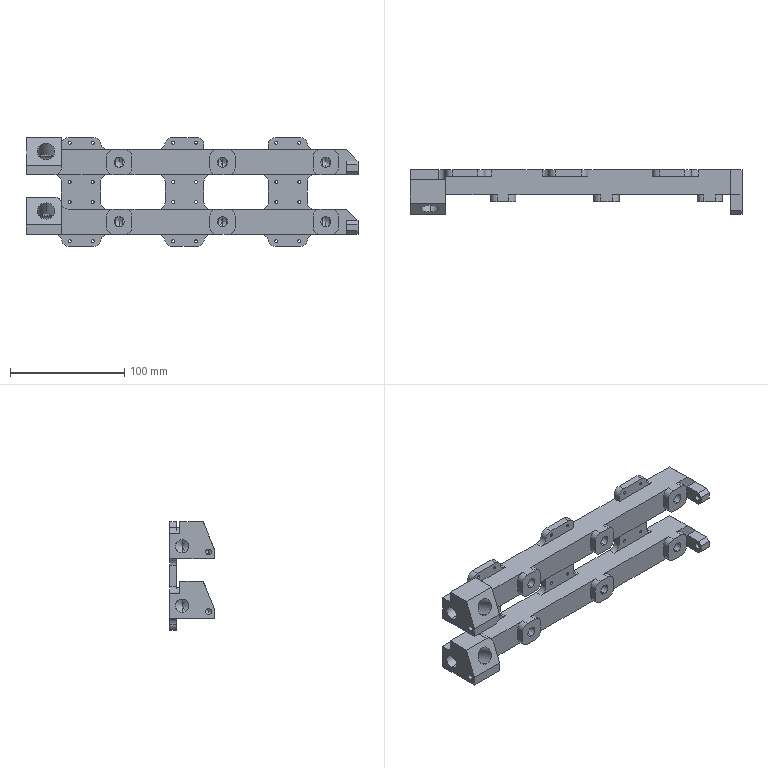NC program | NX | posted by the shop | part box 290 x 39.082 x 95 mm
Lines 26 to 834 of 5678:
(Adaptive-Milling, tool: D16)
N48 M6
N50 G54
N52 G17 G0 G90 X1.222 Y-63.601 S6000 M3
N54 G43 Z30. H0
N56 Z-39.
N58 G94 G1 X1.22 Y-63.551 Z-39.312 F3000.
N60 X1.219 Y-63.501 Z-39.436
N62 X1.218 Y-63.451 Z-39.527
N64 X1.216 Y-63.401 Z-39.6
N66 X1.215 Y-63.351 Z-39.661
N68 X1.214 Y-63.301 Z-39.714
N70 X1.212 Y-63.251 Z-39.76
N72 X1.211 Y-63.201 Z-39.8
N74 X1.209 Y-63.151 Z-39.835
N76 X1.208 Y-63.101 Z-39.866
N78 X1.207 Y-63.051 Z-39.893
N80 X1.205 Y-63.001 Z-39.917
N82 X1.204 Y-62.951 Z-39.937
N84 X1.203 Y-62.901 Z-39.954
N86 X1.201 Y-62.851 Z-39.968
N88 X1.2 Y-62.801 Z-39.98
N90 X1.198 Y-62.751 Z-39.989
N92 X1.197 Y-62.701 Z-39.995
N94 X1.196 Y-62.651 Z-39.999
N96 X1.194 Y-62.601 Z-40.
N98 X1.124 Y-60.047
N100 G3 X0.121 Y-58.596 R1.616
N102 X-2.756 Y-57.933 R10.574
N104 X-10.565 Y-57.551 R79.563
N106 X-23.969 Y-57.499 R842.44
N108 G1 X-143.716 Y-57.497
N110 G2 X-150.412 Y-54.647 R8.844
N112 X-153.599 Y-48.91 R13.945
N114 X-154.723 Y-41.889 R32.079
N116 X-154.983 Y-30.394 R194.097
N118 G1 X-154.996 Y-18.644
N120 Y46.304
N122 G2 X-152.083 Y52.973 R8.856
N124 X-146.325 Y56.123 R14.048
N126 X-139.426 Y57.22 R32.433
N128 X-128.931 Y57.479 R177.832
N130 G1 X-116.431 Y57.496
N132 X143.798
N134 G2 X150.38 Y54.674 R8.82
N136 X153.582 Y48.946 R13.912
N138 X154.719 Y41.927 R31.91
N140 X154.985 Y30.057 R196.37
N142 G1 X154.996 Y19.057
N144 X154.995 Y-46.398
N146 G2 X152.283 Y-52.775 R8.763
N148 X146.592 Y-56.038 R13.714
N150 X139.829 Y-57.19 R30.586
N152 X129.835 Y-57.476 R154.434
N154 G1 X117.71 Y-57.497
N156 X-11.965 Y-57.486
N158 G3 X-16.599 Y-56.761 R20.882
N160 X-26.006 Y-56.52 R167.041
N162 G1 X-37.716 Y-56.498
N164 X-140.466 Y-56.497
N166 G2 X-149.199 Y-52.31 R11.452
N168 X-152.55 Y-45.642 R17.207
N170 X-153.68 Y-38.24 R38.177
N172 X-153.974 Y-26.996 R188.105
N174 G1 X-153.995 Y-15.746
N176 X-153.996 Y42.841
N178 G2 X-153.526 Y46.171 R11.94
N180 G3 X-153.5 Y47.501 R9.579
N182 G1 X-153.395 Y48.831
N184 X-153.084 Y50.128
N186 X-152.573 Y51.36
N188 X-151.876 Y52.497
N190 X-151.01 Y53.511
N192 X-149.995 Y54.377
N194 X-148.858 Y55.074
N196 X-147.625 Y55.584
N198 X-146.329 Y55.895
N200 G2 X-142.608 Y56.081 R66.953
N202 X-124.249 Y56.484 R348.204
N204 G1 X-112.999 Y56.496
N206 X140.458 Y56.495
N208 G2 X149.223 Y52.273 R11.454
N210 X152.53 Y45.699 R17.19
N212 X153.702 Y37.925 R38.906
N214 X153.976 Y26.555 R200.993
N216 G1 X153.994 Y17.78
N218 X153.996 Y-42.833
N220 G2 X149.811 Y-51.692 R11.45
N222 X143.384 Y-54.978 R17.031
N224 X135.867 Y-56.171 R37.276
N226 X124.248 Y-56.48 R186.62
N228 G1 X113.248 Y-56.496
N230 X-11.927 Y-56.485
N232 G3 X-15.509 Y-56. R56.716
N234 G2 X-20.71 Y-55.788 R43.702
N236 G3 X-32.738 Y-55.51 R211.534
N238 G1 X-41.966 Y-55.498
N240 X-81.716
N242 G3 X-83.887 Y-55.893 R35.827
N244 G1 X-85.646 Y-56.
N246 X-107.835
N248 X-112.442 Y-55.682
N250 G3 X-123.727 Y-55.504 R282.665
N252 G1 X-129.467 Y-55.498
N254 G2 X-138.091 Y-55.47 R383.548
N256 X-148.481 Y-49.811 R13.286
N258 X-151.597 Y-42.762 R20.073
N260 G3 X-152.244 Y-41.447 R2.824
N262 G2 X-153.5 Y-36.999 R8.859
N264 G1 Y-4.499
N266 G3 X-153.038 Y5.415 R104.751
N268 G1 X-153.016 Y12.103
N270 G3 X-153.214 Y12.777 R3.314
N272 G1 X-153.461 Y14.041
N274 X-153.5 Y15.
N276 Y47.501
N278 X-153.395 Y48.831
N280 X-153.084 Y50.128
N282 X-152.573 Y51.36
N284 X-151.876 Y52.497
N286 X-151.01 Y53.511
N288 X-149.995 Y54.377
N290 X-148.858 Y55.074
N292 X-147.625 Y55.584
N294 X-146.329 Y55.895
N296 G2 X-144.749 Y56. R57.431
N298 G1 X-114.
N300 X-110.782 Y55.745
N302 G2 X-108.094 Y56. R16.841
N304 G1 X-85.645
N306 G2 X-81.287 Y55.694 R713.21
N308 G3 X-70.648 Y55.506 R248.45
N310 G1 X-62.415 Y55.496
N312 X-21.54 Y55.498
N314 G3 X-19.393 Y55.893 R85.483
N316 G1 X-17.634 Y56.
N318 X4.46
N320 G2 X8.837 Y55.693 R727.431
N322 G3 X20.222 Y55.502 R266.062
N324 G1 X26.71 Y55.496
N326 X68.835 Y55.504
N328 X70.901 Y55.893
N330 X72.66 Y56.
N332 X94.755
N334 G2 X99.091 Y55.695 R696.64
N336 G3 X109.726 Y55.505 R248.916
N338 G1 X118.46 Y55.496
N340 X137.085 Y55.494
N342 G2 X144.051 Y53.812 R13.906
N344 X149.84 Y47.579 R14.675
N346 X152.116 Y40.203 R24.995
N348 X152.867 Y30.74 R71.969
N350 G3 X153.033 Y29.778 R2.227
N352 G1 X153.383 Y28.408
N354 X153.5 Y26.999
N356 X153.498 Y17.083
N358 X153.5 Y14.776
N360 G3 X153.036 Y5.092 R95.967
N362 G1 X152.996 Y-6.586
N364 X153.003 Y-21.96
N366 G3 X153.404 Y-23.674 R35.017
N368 G1 X153.5 Y-25.
N370 Y-37.002
N372 G2 X153.046 Y-41.868 R93.667
N374 X146.881 Y-51.328 R13.741
N376 X139.617 Y-54.258 R21.35
N378 X130.811 Y-55.277 R52.766
N380 X115.939 Y-55.492 R356.297
N382 G1 X109.314 Y-55.495
N384 X98.594 Y-55.502
N386 X96.513 Y-55.893
N388 X94.754 Y-56.
N390 X72.565
N392 X67.934 Y-55.68
N394 G3 X56.4 Y-55.501 R289.681
N396 G1 X50.408 Y-55.496
N398 X8.409 Y-55.502
N400 X6.313 Y-55.893
N402 X4.554 Y-56.
N404 X-15.571
N406 G3 X-17.331 Y-57.76 R1.76
N408 X-15.569 Y-59.52 R1.76
N410 G1 X5.487 Y-59.487
N412 X8.652 Y-59.482 Z-39.9
N414 X68.036 Y-59.387
N416 X70.578 Y-59.379 Z-39.98
N418 G3 X71.182 Y-59.24 Z-40. R1.784
N420 X70.805 Y-55.893 R1.76
N422 G2 X68.041 Y-55.292 R22.211
N424 G3 X62.095 Y-54.676 R36.772
N426 X48.779 Y-54.5 R351.4
N428 G1 X43.284 Y-54.497
N430 X11.705 Y-54.499
N432 G3 X10.661 Y-54.623 R2.926
N434 G1 X9.728 Y-55.045
N436 X8.059 Y-55.569
N438 G3 X7.299 Y-58.449 R1.76
N440 X8.589 Y-59.009 Z-39.954 R1.774
N442 G1 X10.307 Y-59.005 Z-39.9
N444 X66.458 Y-58.903
N446 X67.375 Y-58.904 Z-39.929
N448 X68.292 Y-58.893 Z-39.958
N450 G3 X69.469 Y-58.346 Z-40. R1.759
N452 X68.714 Y-55.46 R1.76
N454 G2 X66.768 Y-54.786 R15.2
N456 G3 X61.979 Y-53.911 R21.369
N458 X51.6 Y-53.532 R135.121
N460 G1 X40.658 Y-53.497
N462 X14.929 Y-53.498
N464 G3 X12.662 Y-53.61 R17.193
N466 G1 X12.243 Y-53.763
N468 G2 X10.651 Y-54.627 R9.276
N470 G3 X9.899 Y-57.184 R1.76
N472 X11.369 Y-57.99 Z-39.945 R1.77
N474 G1 X12.786 Y-57.997 Z-39.9
N476 X64.859 Y-58.246
N478 X66.408 Y-58.248 Z-39.949
N480 G3 X67.77 Y-57.492 Z-40. R1.759
N482 X67.049 Y-54.89 R1.76
N484 X64.569 Y-53.838 R23.295
N486 X59.15 Y-52.916 R26.53
N488 X47.609 Y-52.527 R158.235
N490 G1 X36.659 Y-52.498
N492 X17.925 Y-52.499
N494 G3 X14.061 Y-52.692 R24.817
N496 X13.373 Y-52.978 R2.086
N498 G2 X12.199 Y-53.79 R6.674
N500 G3 X11.578 Y-56.152 R1.76
N502 X13.097 Y-57.053 Z-39.942 R1.77
N504 G1 X14.411 Y-57.066 Z-39.9
N506 X63.502 Y-57.565
N508 X64.227 Y-57.575 Z-39.923
N510 X64.951 Y-57.574 Z-39.946
N512 G3 X66.37 Y-56.738 Z-40. R1.759
N514 X65.785 Y-54.317 R1.76
N516 X61.719 Y-52.622 R10.968
N518 X54.751 Y-51.784 R43.548
N520 X41.639 Y-51.509 R266.83
N522 G1 X32.909 Y-51.498
N524 X20.429 Y-51.499
N526 G3 X15.695 Y-51.706 R35.54
N528 X14.322 Y-52.205 R2.598
N530 G1 X13.339 Y-53.004
N532 G3 X12.885 Y-55.227 R1.76
N534 X14.403 Y-56.145 Z-39.941 R1.768
N536 G1 X15.708 Y-56.166 Z-39.9
N538 X62.424 Y-56.907
N540 X63.149 Y-56.92 Z-39.923
N542 X63.874 Y-56.924 Z-39.946
N544 G3 X65.297 Y-56.097 Z-40. R1.759
N546 X64.717 Y-53.666 R1.76
N548 G2 X63.737 Y-53.003 R15.581
N550 G3 X60.216 Y-51.706 R12.37
N552 X52.864 Y-50.808 R46.008
N554 X40.254 Y-50.517 R250.806
N556 G1 X29.284 Y-50.499
N558 G3 X19.402 Y-50.551 R371.934
N560 X15.879 Y-50.988 R15.225
N562 X15.14 Y-51.379 R1.96
N564 G1 X14.261 Y-52.267
N566 G3 X13.968 Y-54.35 R1.76
N568 X15.473 Y-55.265 Z-39.942 R1.77
N570 G1 X16.793 Y-55.294 Z-39.9
N572 X61.531 Y-56.277
N574 X62.244 Y-56.295 Z-39.923
N576 X62.957 Y-56.303 Z-39.945
N578 G3 X64.397 Y-55.463 Z-40. R1.759
N580 X63.985 Y-53.166 R1.76
N582 X60.172 Y-51.133 R9.407
N584 X53.741 Y-50.023 R33.309
N586 X41.464 Y-49.545 R160.724
N588 X21.591 Y-49.539 R913.993
N590 X17.273 Y-49.958 R23.512
N592 X15.954 Y-50.487 R3.289
N594 X15.462 Y-51.054 R3.39
N596 G1 X15.11 Y-51.409
N598 G3 X14.827 Y-53.51 R1.76
N600 X16.315 Y-54.406 Z-39.943 R1.77
N602 G1 X17.662 Y-54.442 Z-39.9
N604 X60.641 Y-55.574
N606 X61.354 Y-55.594 Z-39.923
N608 X62.067 Y-55.605 Z-39.945
N610 G3 X63.51 Y-54.771 Z-40. R1.759
N612 X63.103 Y-52.468 R1.76
N614 X62.126 Y-51.631 R29.37
N616 X58.514 Y-50.084 R11.955
N618 X51.328 Y-48.973 R40.018
N620 X38.472 Y-48.54 R189.584
N622 X22.867 Y-48.556 R560.146
N624 X18.251 Y-49.017 R26.227
N626 X16.616 Y-49.644 R4.415
N628 G1 X16.389 Y-49.855
N630 X15.701 Y-50.744
N632 G3 X15.586 Y-52.73 R1.76
N634 X17.035 Y-53.58 Z-39.945 R1.77
N636 G1 X18.447 Y-53.627 Z-39.9
N638 X59.98 Y-54.992
N640 X60.703 Y-55.017 Z-39.923
N642 X61.425 Y-55.033 Z-39.946
N644 G3 X62.864 Y-54.226 Z-40. R1.759
N646 X62.633 Y-52.039 R1.76
N648 X59.421 Y-49.831 R7.907
N650 X53.287 Y-48.356 R26.234
N652 X42.607 Y-47.64 R100.888
N654 X24.477 Y-47.56 R476.924
N656 X19.135 Y-48.082 R29.78
N658 X17.238 Y-48.779 R6.156
N660 X16.54 Y-49.659 R2.333
N662 G1 X16.387 Y-49.857
N664 G3 X16.278 Y-51.853 R1.76
N666 X17.716 Y-52.693 Z-39.945 R1.77
N668 G1 X19.145 Y-52.745 Z-39.9
N670 X59.185 Y-54.187
N672 X59.907 Y-54.215 Z-39.923
N674 X60.628 Y-54.234 Z-39.946
N676 G3 X62.071 Y-53.43 Z-40. R1.759
N678 X61.842 Y-51.239 R1.76
N680 X61.021 Y-50.381 R13.833
N682 X57.589 Y-48.604 R10.794
N684 X50.608 Y-47.212 R33.569
N686 X38.296 Y-46.59 R137.151
N688 X27.135 Y-46.545 R869.367
N690 X20.636 Y-47.01 R42.298
N692 X17.81 Y-47.92 R8.824
N694 X17.27 Y-48.433 R2.081
N696 G1 X16.759 Y-49.292
N698 G3 X16.807 Y-51.168 R1.76
N700 X18.198 Y-51.951 Z-39.948 R1.771
N702 G1 X19.704 Y-52.013 Z-39.9
N704 X58.658 Y-53.632
N706 X60.138 Y-53.688 Z-39.947
N708 G3 X61.565 Y-52.924 Z-40. R1.759
N710 X61.504 Y-50.855 R1.76
N712 X58.951 Y-48.648 R6.645
N714 X53.758 Y-46.907 R19.421
N716 X45.109 Y-45.882 R60.777
N718 X26.51 Y-45.608 R264.181
N720 X20.757 Y-46.204 R32.916
N722 X18.084 Y-47.224 R7.939
N724 X17.442 Y-48.145 R1.976
N726 G1 X17.25 Y-48.467
N728 G3 X17.311 Y-50.363 R1.76
N730 X18.682 Y-51.125 Z-39.949 R1.773
N732 G1 X20.219 Y-51.196 Z-39.9
N734 X58.101 Y-52.933
N736 X59.594 Y-52.996 Z-39.947
N738 G3 X61.017 Y-52.25 Z-40. R1.759
N740 X60.969 Y-50.162 R1.76
N742 X58.008 Y-47.664 R7.327
N744 X52.138 Y-45.828 R22.377
N746 G1 X50.108 Y-45.5
N748 X22.233
N750 G3 X18.864 Y-46.276 R8.417
N752 X17.878 Y-47.155 R2.116
N754 G1 X17.576 Y-47.841
N756 G3 X18.129 Y-49.957 R1.76
N758 X19.873 Y-50.171 Z-39.942 R1.77
N760 G1 X21.092 Y-49.655 Z-39.9
N762 X21.552 Y-49.46
N764 X23.003 Y-48.84 Z-39.95
N766 G3 X23.952 Y-47.636 Z-40. R1.759
N768 X22.233 Y-45.5 R1.76
N770 X20.258 Y-45.527 R23.231
N772 X18.459 Y-46.204 R3.403
N774 X17.878 Y-47.155 R2.329
N776 X20.326 Y-49.413 R1.76
N778 G1 X21.444 Y-48.808
N780 G3 X20.608 Y-45.5 R1.76
N782 X19.437 Y-45.532 R10.983
N784 X18.07 Y-46.721 R1.795
N786 X19.541 Y-49.185 R1.76
N788 G1 X19.792 Y-49.205
N790 X22.946 Y-49.455 Z-39.9
N792 X57.538 Y-52.202
N794 X59.025 Y-52.315 Z-39.947
N796 G3 X60.474 Y-51.614 Z-40. R1.759
N798 X60.579 Y-49.658 R1.76
N800 X58.535 Y-47.483 R5.64
N802 X53.884 Y-45.511 R15.642
N804 G1 X50.011 Y-45.5
N806 G3 X48.436 Y-48.047 R1.76
N808 X49.496 Y-48.943 Z-39.955 R1.778
N810 G1 X51.158 Y-49.452 Z-39.9
N812 X56.884 Y-51.204
N814 X57.574 Y-51.417 Z-39.923
N816 X58.266 Y-51.62 Z-39.946
N818 G3 X59.868 Y-51.215 Z-40. R1.759
N820 X60.195 Y-49.013 R1.76
N822 X57.952 Y-46.628 R6.173
N824 X55.898 Y-45.558 R10.323
N826 G1 X55.549 Y-45.5
N828 X53.674
N830 G3 X51.944 Y-47.584 R1.76
N832 X52.973 Y-48.874 Z-39.946 R1.77
N834 G1 X54.301 Y-49.451 Z-39.9
N836 X56.382 Y-50.355
N838 X57.036 Y-50.641 Z-39.923
N840 X57.694 Y-50.918 Z-39.945
N842 G3 X59.343 Y-50.686 Z-40. R1.759
N844 X59.812 Y-48.369 R1.76
N846 X59.213 Y-47.363 R8.452
N848 X57.102 Y-45.626 R6.695
N850 X56.564 Y-45.5 R3.835
N852 G1 X55.439
N854 G3 X53.681 Y-47.34 R1.76
N856 X54.603 Y-48.809 Z-39.943 R1.77
N858 G1 X55.791 Y-49.45 Z-39.9
N860 X55.963 Y-49.543
N862 X56.59 Y-49.884 Z-39.923
N864 X57.222 Y-50.216 Z-39.945
N866 G3 X58.885 Y-50.125 Z-40. R1.759
N868 X59.576 Y-47.914 R1.76
N870 X57.868 Y-45.718 R4.353
N872 X57.147 Y-45.5 R2.125
N874 G1 X56.522
N876 G3 X55.548 Y-48.726 R1.76
N878 G1 X56.739 Y-49.518
N880 G3 X59.324 Y-47.342 R1.76
N882 X58.665 Y-46.109 R4.449
N884 X57.102 Y-45.5 R1.839
N886 X56.962 Y-49.014 R1.76
N888 X57.62 Y-49.023 R2.67
N890 X58.943 Y-46.493 R1.76
N892 X57.729 Y-45.544 R1.681
N894 X56.071 Y-46.236 R1.6
N896 G1 X55.7 Y-46.803
N898 X53.968 Y-49.452 Z-39.9
N900 X53.777 Y-49.747
N902 X53.576 Y-50.035
N904 G2 X52.694 Y-50.578 R1.604
N906 G1 X13.152 Y-59.545
N908 G2 X6.139 Y-60.595 R49.098
N910 X1.411 Y-60.803 R66.372
N912 G1 X-14.36 Y-60.928
N914 G2 X-15.666 Y-60.269 R1.601
N916 G1 X-15.887 Y-59.966
N918 X-17.749 Y-57.407 Z-40.
N920 X-18.119 Y-56.894
N922 X-18.501 Y-56.39
N924 G3 X-19.395 Y-55.893 R1.604
N926 G2 X-22.115 Y-55.306 R22.564
N928 G3 X-28.157 Y-54.683 R37.988
N930 X-41.472 Y-54.501 R350.861
N932 G1 X-46.966 Y-54.498
N934 X-77.347 Y-54.501
N936 G3 X-79.234 Y-54.538 R19.473
N938 X-80.472 Y-55.045 R6.456
N940 G1 X-82.141 Y-55.569
N942 G3 X-82.901 Y-58.449 R1.76
N944 X-81.611 Y-59.009 Z-39.954 R1.774
N946 G1 X-79.893 Y-59.005 Z-39.9
N948 X-23.742 Y-58.903
N950 X-22.825 Y-58.904 Z-39.929
N952 X-21.908 Y-58.893 Z-39.958
N954 G3 X-20.731 Y-58.346 Z-40. R1.759
N956 X-21.486 Y-55.46 R1.76
N958 G2 X-23.664 Y-54.716 R28.096
N960 G3 X-28.812 Y-53.867 R24.602
N962 X-40.008 Y-53.523 R164.268
N964 G1 X-49.467 Y-53.499
N966 X-74.954 Y-53.5
N968 G3 X-77.526 Y-53.608 R19.433
N970 G1 X-77.964 Y-53.767
N972 G2 X-79.549 Y-54.627 R9.223
N974 G3 X-80.303 Y-57.182 R1.76
N976 X-78.833 Y-57.99 Z-39.945 R1.77
N978 G1 X-77.417 Y-57.998 Z-39.9
N980 X-25.23 Y-58.296
N982 X-23.68 Y-58.3 Z-39.949
N984 G3 X-22.318 Y-57.546 Z-40. R1.759
N986 X-23.038 Y-54.941 R1.76
N988 X-25.593 Y-53.855 R24.387
N990 X-31.096 Y-52.918 R26.592
N992 X-42.642 Y-52.529 R159.475
N994 G1 X-53.591 Y-52.5
N996 X-72.329
N998 G3 X-76.143 Y-52.69 R24.466
N1000 X-76.829 Y-52.979 R2.071
N1002 G2 X-78.001 Y-53.79 R6.668
N1004 G3 X-78.622 Y-56.152 R1.76
N1006 X-77.103 Y-57.053 Z-39.942 R1.77
N1008 G1 X-75.789 Y-57.066 Z-39.9
N1010 X-26.698 Y-57.565
N1012 X-25.973 Y-57.575 Z-39.923
N1014 X-25.249 Y-57.574 Z-39.946
N1016 G3 X-23.83 Y-56.738 Z-40. R1.759
N1018 X-24.415 Y-54.317 R1.76
N1020 X-28.515 Y-52.619 R11.014
N1022 X-35.847 Y-51.767 R46.047
N1024 X-48.86 Y-51.511 R279.995
N1026 G1 X-57.091 Y-51.5
N1028 X-69.821
N1030 G3 X-74.454 Y-51.694 R37.434
N1032 X-75.745 Y-52.102 R2.868
N1034 G1 X-76.861 Y-53.004
N1036 G3 X-77.315 Y-55.227 R1.76
N1038 X-75.797 Y-56.145 Z-39.941 R1.768
N1040 G1 X-74.492 Y-56.166 Z-39.9
N1042 X-27.776 Y-56.907
N1044 X-27.051 Y-56.92 Z-39.923
N1046 X-26.326 Y-56.924 Z-39.946
N1048 G3 X-24.903 Y-56.097 Z-40. R1.759
N1050 X-25.483 Y-53.666 R1.76
N1052 G2 X-26.475 Y-52.998 R17.673
N1054 G3 X-30.03 Y-51.707 R12.304
N1056 X-37.385 Y-50.81 R46.137
N1058 X-49.748 Y-50.52 R247.617
N1060 G1 X-60.716 Y-50.5
N1062 G3 X-70.96 Y-50.557 R352.894
N1064 X-74.413 Y-51.014 R13.98
N1066 X-75.061 Y-51.38 R2.092
N1068 G1 X-75.941 Y-52.269
N1070 G3 X-76.233 Y-54.352 R1.76
N1072 X-74.728 Y-55.266 Z-39.942 R1.77
N1074 G1 X-73.408 Y-55.295 Z-39.9
N1076 X-28.669 Y-56.277
N1078 X-27.956 Y-56.295 Z-39.923
N1080 X-27.243 Y-56.303 Z-39.945
N1082 G3 X-25.803 Y-55.463 Z-40. R1.759
N1084 X-26.215 Y-53.166 R1.76
N1086 X-29.81 Y-51.207 R9.157
N1088 X-36.283 Y-50.044 R32.125
N1090 X-47.678 Y-49.56 R147.388
N1092 X-68.429 Y-49.535 R947.944
N1094 X-72.881 Y-49.948 R24.433
N1096 X-74.16 Y-50.419 R3.602
N1098 X-74.738 Y-51.054 R2.735
N1100 G1 X-75.09 Y-51.409
N1102 G3 X-75.373 Y-53.51 R1.76
N1104 X-73.885 Y-54.406 Z-39.943 R1.77
N1106 G1 X-72.538 Y-54.442 Z-39.9
N1108 X-29.559 Y-55.574
N1110 X-28.846 Y-55.594 Z-39.923
N1112 X-28.133 Y-55.605 Z-39.945
N1114 G3 X-26.69 Y-54.771 Z-40. R1.759
N1116 X-27.097 Y-52.468 R1.76
N1118 G1 X-27.826 Y-51.819
N1120 G3 X-31.282 Y-50.205 R10.652
N1122 X-38.125 Y-49.041 R36.074
N1124 X-50.419 Y-48.555 R163.69
N1126 X-67.151 Y-48.55 R638.118
N1128 X-71.823 Y-48.989 R27.96
N1130 X-73.496 Y-49.576 R5.152
N1132 G1 X-73.802 Y-49.844
N1134 X-74.491 Y-50.734
N1136 G3 X-74.606 Y-52.72 R1.76
N1138 X-73.157 Y-53.57 Z-39.945 R1.77
N1140 G1 X-71.744 Y-53.617 Z-39.9
N1142 X-30.22 Y-54.991
N1144 X-29.498 Y-55.017 Z-39.923
N1146 X-28.775 Y-55.033 Z-39.946
N1148 G3 X-27.336 Y-54.226 Z-40. R1.759
N1150 X-27.567 Y-52.039 R1.76
N1152 X-30.965 Y-49.763 R8.15
N1154 X-36.956 Y-48.354 R26.561
N1156 X-47.643 Y-47.641 R101.61
N1158 X-65.771 Y-47.562 R474.164
N1160 X-70.841 Y-48.034 R31.056
N1162 X-72.896 Y-48.729 R7.396
N1164 X-73.66 Y-49.659 R2.443
N1166 G1 X-73.813 Y-49.857
N1168 G3 X-73.923 Y-51.851 R1.76
N1170 X-72.487 Y-52.693 Z-39.945 R1.77
N1172 G1 X-71.057 Y-52.747 Z-39.9
N1174 X-30.93 Y-54.273
N1176 X-30.209 Y-54.303 Z-39.923
N1178 X-29.487 Y-54.323 Z-39.946
N1180 G3 X-28.043 Y-53.521 Z-40. R1.759
N1182 X-28.27 Y-51.328 R1.76
N1184 X-29.169 Y-50.392 R19.909
N1186 X-32.507 Y-48.643 R10.573
N1188 X-39.192 Y-47.261 R32.278
N1190 X-51.341 Y-46.602 R128.298
N1192 X-63.468 Y-46.553 R704.361
N1194 X-69.509 Y-47.002 R41.449
N1196 X-72.376 Y-47.905 R9.1
N1198 X-72.919 Y-48.415 R2.1
N1200 G1 X-73.431 Y-49.275
N1202 G3 X-73.382 Y-51.151 R1.76
N1204 X-71.992 Y-51.933 Z-39.948 R1.771
N1206 G1 X-70.484 Y-51.996 Z-39.9
N1208 X-31.542 Y-53.632
N1210 X-30.063 Y-53.688 Z-39.947
N1212 G3 X-28.635 Y-52.925 Z-40. R1.759
N1214 X-28.696 Y-50.855 R1.76
N1216 X-31.275 Y-48.636 R6.662
N1218 X-36.893 Y-46.821 R20.822
N1220 X-46.202 Y-45.823 R68.664
N1222 X-63.851 Y-45.616 R267.848
N1224 X-69.478 Y-46.212 R32.459
N1226 X-72.13 Y-47.233 R7.706
N1228 X-72.758 Y-48.145 R1.994
N1230 G1 X-72.95 Y-48.467
N1232 G3 X-72.889 Y-50.363 R1.76
N1234 X-71.518 Y-51.125 Z-39.949 R1.773
N1236 G1 X-69.981 Y-51.196 Z-39.9
N1238 X-32.099 Y-52.933
N1240 X-30.606 Y-52.996 Z-39.947
N1242 G3 X-29.183 Y-52.25 Z-40. R1.759
N1244 X-29.231 Y-50.162 R1.76
N1246 X-31.865 Y-47.841 R6.959
N1248 X-37.478 Y-45.949 R20.618
N1250 X-40.132 Y-45.5 R59.726
N1252 G1 X-68.175 Y-45.513
N1254 G3 X-71.649 Y-46.448 R7.718
N1256 X-72.326 Y-47.165 R1.84
N1258 G1 X-72.629 Y-47.851
N1260 G3 X-72.085 Y-49.961 R1.76
N1262 X-70.344 Y-50.187 Z-39.942 R1.77
N1264 G1 X-69.118 Y-49.678 Z-39.9
N1266 X-68.591 Y-49.46
N1268 X-67.124 Y-48.846 Z-39.95
N1270 G3 X-66.168 Y-47.662 Z-40. R1.759
N1272 X-67.882 Y-45.5 R1.76
N1274 X-69.935 Y-45.524 R28.585
N1276 X-71.717 Y-46.179 R3.457
N1278 X-72.36 Y-47.241 R2.727
N1280 X-69.824 Y-49.448 R1.76
N1282 G1 X-68.706 Y-48.757
N1284 G3 X-69.632 Y-45.5 R1.76
N1286 X-70.763 Y-45.532 R10.852
N1288 X-72.13 Y-46.721 R1.795
N1290 X-70.659 Y-49.185 R1.76
N1292 G1 X-70.408 Y-49.205
N1294 X-67.254 Y-49.455 Z-39.9
N1296 X-32.662 Y-52.202
N1298 X-31.175 Y-52.315 Z-39.947
N1300 G3 X-29.726 Y-51.614 Z-40. R1.759
N1302 X-29.621 Y-49.658 R1.76
N1304 X-31.815 Y-47.391 R5.887
N1306 X-36.353 Y-45.508 R15.701
N1308 G1 X-40.195 Y-45.5
N1310 G3 X-41.791 Y-48.002 R1.76
N1312 X-40.725 Y-48.938 Z-39.954 R1.773
N1314 G1 X-39.099 Y-49.452 Z-39.9
N1316 X-33.261 Y-51.296
N1318 X-32.574 Y-51.514 Z-39.923
N1320 X-31.885 Y-51.724 Z-39.946
N1322 G3 X-30.278 Y-51.331 Z-40. R1.759
N1324 X-29.941 Y-49.121 R1.76
N1326 X-32.273 Y-46.615 R6.291
N1328 X-34.332 Y-45.553 R9.809
N1330 G1 X-34.651 Y-45.5
N1332 X-36.526
N1334 G3 X-38.256 Y-47.584 R1.76
N1336 X-37.227 Y-48.874 Z-39.946 R1.77
N1338 G1 X-35.9 Y-49.451 Z-39.9
N1340 X-33.818 Y-50.355
N1342 X-33.164 Y-50.641 Z-39.923
N1344 X-32.506 Y-50.918 Z-39.945
N1346 G3 X-30.857 Y-50.686 Z-40. R1.759
N1348 X-30.388 Y-48.369 R1.76
N1350 X-30.99 Y-47.361 R8.305
N1352 X-33.15 Y-45.613 R6.41
N1354 X-33.645 Y-45.5 R7.782
N1356 G1 X-34.77
N1358 G3 X-36.528 Y-47.343 R1.76
N1360 X-35.604 Y-48.81 Z-39.943 R1.77
N1362 G1 X-34.413 Y-49.45 Z-39.9
N1364 X-34.236 Y-49.546
N1366 X-33.608 Y-49.886 Z-39.923
N1368 X-32.975 Y-50.217 Z-39.945
N1370 G3 X-31.313 Y-50.124 Z-40. R1.759
N1372 X-30.624 Y-47.914 R1.76
N1374 X-32.343 Y-45.716 R4.342
N1376 X-33.06 Y-45.5 R2.139
N1378 G1 X-33.685
N1380 G3 X-34.655 Y-48.728 R1.76
N1382 G1 X-33.457 Y-49.52
N1384 G3 X-30.876 Y-47.342 R1.76
N1386 X-31.696 Y-45.956 R3.954
N1388 X-33.098 Y-45.5 R1.858
N1390 X-33.669 Y-48.925 R1.76
N1392 G1 X-33.418 Y-49.01
N1394 X-33.164 Y-49.086
N1396 G3 X-31.178 Y-46.656 R1.76
N1398 X-32.586 Y-45.521 R1.758
N1400 X-34. Y-46.186 R1.601
N1402 G1 X-34.494 Y-46.878
N1404 X-36.334 Y-49.452 Z-39.9
N1406 X-36.557 Y-49.769
N1408 X-36.795 Y-50.076
N1410 G2 X-37.62 Y-50.556 R1.606
N1412 G1 X-77.163 Y-59.523
N1414 G2 X-84.176 Y-60.575 R49.295
N1416 X-88.904 Y-60.787 R66.833
N1418 G1 X-104.56 Y-60.928
N1420 G2 X-105.868 Y-60.269 R1.601
N1422 G1 X-106.089 Y-59.965
N1424 X-107.95 Y-57.406 Z-40.
N1426 X-108.319 Y-56.893
N1428 X-108.701 Y-56.39
N1430 G3 X-109.595 Y-55.893 R1.604
N1432 G2 X-112.343 Y-55.296 R21.655
N1434 G3 X-118.281 Y-54.678 R36.613
N1436 X-131.596 Y-54.501 R351.169
N1438 G2 X-136.591 Y-54.388 R56.282
N1440 X-147.561 Y-47.771 R14.554
N1442 X-149.504 Y-44.354 R46.844
N1444 G3 X-149.863 Y-43.971 R3.099
N1446 G2 X-151.555 Y-42.411 R9.77
N1448 G1 X-151.919 Y-41.902
N1450 G3 X-154.503 Y-41.876 R1.6
N1452 X-154.791 Y-43.175 Z-39.957 R1.678
N1454 G1 X-154.572 Y-44.957 Z-39.9
N1456 X-154.218 Y-47.844
N1458 G3 X-153.762 Y-48.78 R1.604
N1460 G1 X-148.167 Y-54.375
N1462 G3 X-144.454 Y-57.032 R14.335
N1464 X-139.781 Y-58.694 R19.135
N1466 X-137.554 Y-59.003 R17.199
N1468 G1 X-116.721 Y-60.495
N1470 G3 X-115.974 Y-60.369 R1.615
N1472 G1 X-113.159 Y-59.157
N1474 X-111.454 Y-58.418 Z-39.959
N1476 G3 X-110.633 Y-57.449 Z-40. R1.6
N1478 X-111.686 Y-55.46 R1.6
N1480 G2 X-113.841 Y-54.721 R25.579
N1482 G3 X-118.944 Y-53.867 R23.876
N1484 X-128.776 Y-53.534 R146.543
N1486 G2 X-134.256 Y-53.398 R76.692
N1488 X-145.17 Y-47.951 R15.791
N1490 G3 X-147.511 Y-45.243 R118.595
N1492 G1 X-147.873 Y-45.
N1494 G2 X-149.863 Y-43.971 R9.861
N1496 G3 X-152.087 Y-44.561 R1.6
N1498 X-152.186 Y-45.91 Z-39.956 R1.612
N1500 G1 X-151.557 Y-47.562 Z-39.9
N1502 X-150.922 Y-49.232
N1504 G3 X-149.863 Y-50.202 R1.601
N1506 G1 X-117.643 Y-59.347
N1508 G3 X-116.579 Y-59.28 R1.604
N1510 G1 X-114.877 Y-58.554
N1512 X-113.192 Y-57.831 Z-39.958
N1514 G3 X-112.361 Y-56.842 Z-40. R1.6
N1516 X-113.238 Y-54.941 R1.6
N1518 X-115.896 Y-53.818 R23.517
N1520 X-121.445 Y-52.899 R27.382
N1522 X-130.373 Y-52.533 R170.135
N1524 G2 X-136.649 Y-51.55 R22.314
N1526 X-142.989 Y-47.858 R18.914
N1528 G3 X-145.683 Y-45.615 R45.331
N1530 X-146.793 Y-45.309 R2.868
N1532 G1 X-147.987 Y-44.95
N1534 G3 X-149.163 Y-48.259 R-1.76
N1536 G1 X-147.938 Y-48.601
N1538 X-144.89 Y-49.452 Z-39.9
N1540 X-117.799 Y-57.014
N1542 X-115.914 Y-57.535 Z-39.962
N1544 G3 X-114.738 Y-57.39 Z-40. R1.76
N1546 X-114.615 Y-54.317 R1.76
N1548 X-118.661 Y-52.626 R10.935
N1550 X-125.283 Y-51.806 R42.262
N1552 G2 X-131.188 Y-51.394 R94.331
N1554 X-140.48 Y-47.912 R21.35
N1556 G3 X-143.512 Y-45.931 R97.286
N1558 X-145. Y-45.5 R2.358
N1560 G2 X-146.272 Y-45.392 R8.393
N1562 G3 X-147.681 Y-48.48 R1.76
N1564 X-146.863 Y-48.869 Z-39.971 R1.939
N1566 G1 X-144.69 Y-49.452 Z-39.9
N1568 X-118.667 Y-56.436
N1570 X-116.964 Y-56.888 Z-39.956
N1572 G3 X-115.623 Y-56.633 Z-40. R1.76
N1574 X-115.683 Y-53.666 R1.76
N1576 G2 X-116.703 Y-52.98 R20.85
N1578 G3 X-120.484 Y-51.642 R12.802
N1580 X-125.638 Y-50.926 R45.391
N1582 G2 X-131.695 Y-50.111 R47.179
N1584 X-139.113 Y-47.19 R27.97
N1586 G3 X-142.234 Y-45.594 R34.082
N1588 G1 X-142.7 Y-45.5
N1590 X-144.7
N1592 G3 X-146.16 Y-48.243 R1.76
N1594 X-145.014 Y-48.998 Z-39.956 R1.839
N1596 G1 X-143.317 Y-49.453 Z-39.9
N1598 X-119.387 Y-55.865
N1600 X-117.87 Y-56.266 Z-39.95
N1602 G3 X-116.375 Y-55.895 Z-40. R1.759
N1604 X-116.415 Y-53.166 R1.76
N1606 X-120.211 Y-51.139 R9.375
N1608 X-124.913 Y-50.177 R33.375
N1610 G2 X-131.408 Y-48.952 R53.097
N1612 X-138.214 Y-46.321 R42.873
N1614 G3 X-140.065 Y-45.549 R26.512
N1616 G1 X-140.364 Y-45.5
N1618 X-142.739
N1620 G3 X-144.209 Y-48.228 R1.76
N1622 X-143.047 Y-49. Z-39.955 R1.847
N1624 G1 X-141.374 Y-49.453 Z-39.9
N1626 X-120.225 Y-55.175
N1628 X-118.754 Y-55.568 Z-39.948
N1630 G3 X-117.224 Y-55.168 Z-40. R1.759
N1632 X-117.297 Y-52.468 R1.76
N1634 G1 X-118.029 Y-51.815
N1636 G3 X-121.283 Y-50.257 R10.435
N1638 X-126.697 Y-48.979 R63.74
N1640 G2 X-136.262 Y-45.962 R53.575
N1642 G3 X-137.694 Y-45.5 R6.013
N1644 G1 X-140.444
N1646 G3 X-141.95 Y-48.172 R1.76
N1648 X-140.772 Y-48.996 Z-39.953 R1.843
N1650 G1 X-139.148 Y-49.452 Z-39.9
N1652 X-120.805 Y-54.603
N1654 X-119.396 Y-54.993 Z-39.946
N1656 G3 X-117.817 Y-54.563 Z-40. R1.759
N1658 X-117.767 Y-52.039 R1.76